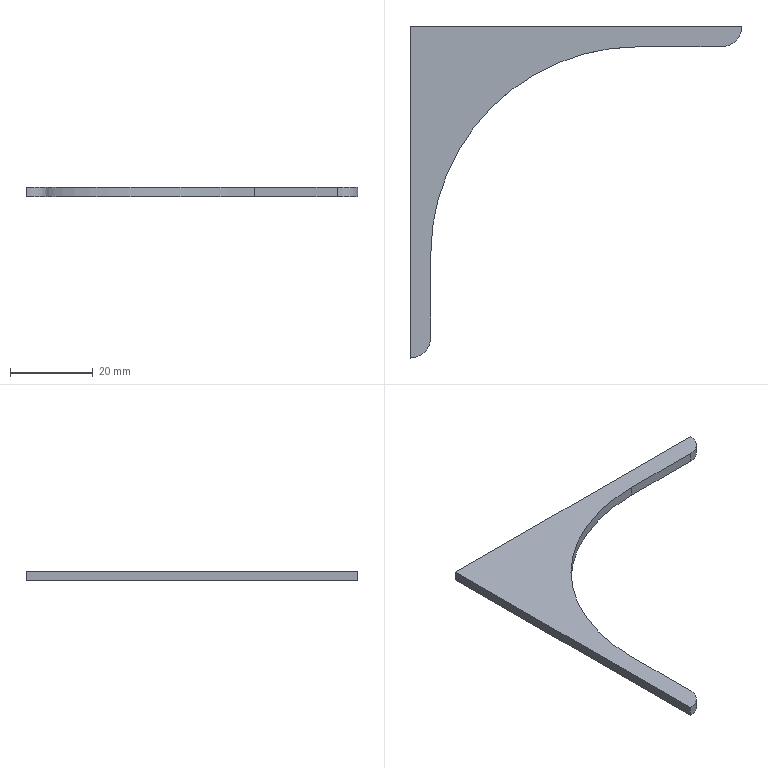Part | SolidWorks | features Fillet 1, FlatPattern 1, SMBaseFlange 1, SheetMetal 1 | 1 solid | 9 faces | box 80 x 80 x 2.3 mm | volume 2992 mm3 | plane 6 | cylinder 3 | commonest cylinder face diameters 10 x2 100 x1
STEP:
#1=CARTESIAN_POINT('',(0.,0.,0.));
#2=VERTEX_POINT('',#1);
#3=CARTESIAN_POINT('',(0.,-80.,0.));
#4=VERTEX_POINT('',#3);
#5=CARTESIAN_POINT('',(0.,0.,0.));
#6=DIRECTION('',(0.,-1.,0.));
#7=VECTOR('',#6,1000.);
#8=LINE('',#5,#7);
#9=EDGE_CURVE('',#2,#4,#8,.T.);
#10=ORIENTED_EDGE('',*,*,#9,.T.);
#11=CARTESIAN_POINT('',(0.,-80.,2.3));
#12=VERTEX_POINT('',#11);
#13=CARTESIAN_POINT('',(0.,-80.,2.3));
#14=DIRECTION('',(0.,0.,-1.));
#15=VECTOR('',#14,1000.);
#16=LINE('',#13,#15);
#17=EDGE_CURVE('',#12,#4,#16,.T.);
#18=ORIENTED_EDGE('',*,*,#17,.F.);
#19=CARTESIAN_POINT('',(0.,0.,2.3));
#20=VERTEX_POINT('',#19);
#21=CARTESIAN_POINT('',(0.,0.,2.3));
#22=DIRECTION('',(0.,-1.,0.));
#23=VECTOR('',#22,1000.);
#24=LINE('',#21,#23);
#25=EDGE_CURVE('',#20,#12,#24,.T.);
#26=ORIENTED_EDGE('',*,*,#25,.F.);
#27=CARTESIAN_POINT('',(0.,0.,2.3));
#28=DIRECTION('',(0.,0.,-1.));
#29=VECTOR('',#28,1000.);
#30=LINE('',#27,#29);
#31=EDGE_CURVE('',#20,#2,#30,.T.);
#32=ORIENTED_EDGE('',*,*,#31,.T.);
#33=EDGE_LOOP('',(#10,#18,#26,#32));
#34=FACE_OUTER_BOUND('',#33,.T.);
#35=CARTESIAN_POINT('',(0.,0.,2.3));
#36=DIRECTION('',(1.,0.,0.));
#37=DIRECTION('',(0.,1.,0.));
#38=AXIS2_PLACEMENT_3D('',#35,#36,#37);
#39=PLANE('',#38);
#40=ADVANCED_FACE('',(#34),#39,.F.);
#41=CARTESIAN_POINT('',(5.,-75.,2.3));
#42=VERTEX_POINT('',#41);
#43=CARTESIAN_POINT('',(5.,-55.,2.3));
#44=VERTEX_POINT('',#43);
#45=CARTESIAN_POINT('',(5.,-80.,2.3));
#46=DIRECTION('',(0.,1.,0.));
#47=VECTOR('',#46,1000.);
#48=LINE('',#45,#47);
#49=EDGE_CURVE('',#42,#44,#48,.T.);
#50=ORIENTED_EDGE('',*,*,#49,.F.);
#51=CARTESIAN_POINT('',(5.,-75.,0.));
#52=VERTEX_POINT('',#51);
#53=CARTESIAN_POINT('',(5.,-75.,2.3));
#54=DIRECTION('',(0.,0.,-1.));
#55=VECTOR('',#54,1000.);
#56=LINE('',#53,#55);
#57=EDGE_CURVE('',#42,#52,#56,.T.);
#58=ORIENTED_EDGE('',*,*,#57,.T.);
#59=CARTESIAN_POINT('',(5.,-55.,0.));
#60=VERTEX_POINT('',#59);
#61=CARTESIAN_POINT('',(5.,-80.,0.));
#62=DIRECTION('',(0.,1.,0.));
#63=VECTOR('',#62,1000.);
#64=LINE('',#61,#63);
#65=EDGE_CURVE('',#52,#60,#64,.T.);
#66=ORIENTED_EDGE('',*,*,#65,.T.);
#67=CARTESIAN_POINT('',(5.,-55.,2.3));
#68=DIRECTION('',(0.,0.,-1.));
#69=VECTOR('',#68,1000.);
#70=LINE('',#67,#69);
#71=EDGE_CURVE('',#44,#60,#70,.T.);
#72=ORIENTED_EDGE('',*,*,#71,.F.);
#73=EDGE_LOOP('',(#50,#58,#66,#72));
#74=FACE_OUTER_BOUND('',#73,.T.);
#75=CARTESIAN_POINT('',(5.,-80.,2.3));
#76=DIRECTION('',(-1.,0.,0.));
#77=DIRECTION('',(0.,-1.,0.));
#78=AXIS2_PLACEMENT_3D('',#75,#76,#77);
#79=PLANE('',#78);
#80=ADVANCED_FACE('',(#74),#79,.F.);
#81=CARTESIAN_POINT('',(55.,-5.,0.));
#82=VERTEX_POINT('',#81);
#83=CARTESIAN_POINT('',(55.,-55.,0.));
#84=DIRECTION('',(0.,0.,-1.));
#85=DIRECTION('',(-1.,0.,0.));
#86=AXIS2_PLACEMENT_3D('',#83,#84,#85);
#87=CIRCLE('',#86,50.);
#88=EDGE_CURVE('',#60,#82,#87,.T.);
#89=ORIENTED_EDGE('',*,*,#88,.T.);
#90=CARTESIAN_POINT('',(55.,-5.,2.3));
#91=VERTEX_POINT('',#90);
#92=CARTESIAN_POINT('',(55.,-5.,2.3));
#93=DIRECTION('',(0.,0.,-1.));
#94=VECTOR('',#93,1000.);
#95=LINE('',#92,#94);
#96=EDGE_CURVE('',#91,#82,#95,.T.);
#97=ORIENTED_EDGE('',*,*,#96,.F.);
#98=CARTESIAN_POINT('',(55.,-55.,2.3));
#99=DIRECTION('',(0.,0.,-1.));
#100=DIRECTION('',(-1.,0.,0.));
#101=AXIS2_PLACEMENT_3D('',#98,#99,#100);
#102=CIRCLE('',#101,50.);
#103=EDGE_CURVE('',#44,#91,#102,.T.);
#104=ORIENTED_EDGE('',*,*,#103,.F.);
#105=ORIENTED_EDGE('',*,*,#71,.T.);
#106=EDGE_LOOP('',(#89,#97,#104,#105));
#107=FACE_OUTER_BOUND('',#106,.T.);
#108=CARTESIAN_POINT('',(55.,-55.,2.3));
#109=DIRECTION('',(0.,0.,-1.));
#110=DIRECTION('',(-1.,0.,0.));
#111=AXIS2_PLACEMENT_3D('',#108,#109,#110);
#112=CYLINDRICAL_SURFACE('',#111,50.);
#113=ADVANCED_FACE('',(#107),#112,.F.);
#114=CARTESIAN_POINT('',(75.,-5.,0.));
#115=VERTEX_POINT('',#114);
#116=CARTESIAN_POINT('',(80.,-5.,0.));
#117=DIRECTION('',(1.,0.,0.));
#118=VECTOR('',#117,1000.);
#119=LINE('',#116,#118);
#120=EDGE_CURVE('',#82,#115,#119,.T.);
#121=ORIENTED_EDGE('',*,*,#120,.T.);
#122=CARTESIAN_POINT('',(75.,-5.,2.3));
#123=VERTEX_POINT('',#122);
#124=CARTESIAN_POINT('',(75.,-5.,2.3));
#125=DIRECTION('',(0.,0.,1.));
#126=VECTOR('',#125,1000.);
#127=LINE('',#124,#126);
#128=EDGE_CURVE('',#115,#123,#127,.T.);
#129=ORIENTED_EDGE('',*,*,#128,.T.);
#130=CARTESIAN_POINT('',(80.,-5.,2.3));
#131=DIRECTION('',(1.,0.,0.));
#132=VECTOR('',#131,1000.);
#133=LINE('',#130,#132);
#134=EDGE_CURVE('',#91,#123,#133,.T.);
#135=ORIENTED_EDGE('',*,*,#134,.F.);
#136=ORIENTED_EDGE('',*,*,#96,.T.);
#137=EDGE_LOOP('',(#121,#129,#135,#136));
#138=FACE_OUTER_BOUND('',#137,.T.);
#139=CARTESIAN_POINT('',(80.,-5.,2.3));
#140=DIRECTION('',(0.,1.,0.));
#141=DIRECTION('',(-1.,0.,0.));
#142=AXIS2_PLACEMENT_3D('',#139,#140,#141);
#143=PLANE('',#142);
#144=ADVANCED_FACE('',(#138),#143,.F.);
#145=CARTESIAN_POINT('',(80.,0.,0.));
#146=VERTEX_POINT('',#145);
#147=CARTESIAN_POINT('',(0.,0.,0.));
#148=DIRECTION('',(-1.,0.,0.));
#149=VECTOR('',#148,1000.);
#150=LINE('',#147,#149);
#151=EDGE_CURVE('',#146,#2,#150,.T.);
#152=ORIENTED_EDGE('',*,*,#151,.T.);
#153=ORIENTED_EDGE('',*,*,#31,.F.);
#154=CARTESIAN_POINT('',(80.,0.,2.3));
#155=VERTEX_POINT('',#154);
#156=CARTESIAN_POINT('',(0.,0.,2.3));
#157=DIRECTION('',(-1.,0.,0.));
#158=VECTOR('',#157,1000.);
#159=LINE('',#156,#158);
#160=EDGE_CURVE('',#155,#20,#159,.T.);
#161=ORIENTED_EDGE('',*,*,#160,.F.);
#162=CARTESIAN_POINT('',(80.,0.,2.3));
#163=DIRECTION('',(0.,0.,-1.));
#164=VECTOR('',#163,1000.);
#165=LINE('',#162,#164);
#166=EDGE_CURVE('',#155,#146,#165,.T.);
#167=ORIENTED_EDGE('',*,*,#166,.T.);
#168=EDGE_LOOP('',(#152,#153,#161,#167));
#169=FACE_OUTER_BOUND('',#168,.T.);
#170=CARTESIAN_POINT('',(0.,0.,2.3));
#171=DIRECTION('',(0.,-1.,0.));
#172=DIRECTION('',(0.,0.,-1.));
#173=AXIS2_PLACEMENT_3D('',#170,#171,#172);
#174=PLANE('',#173);
#175=ADVANCED_FACE('',(#169),#174,.F.);
#176=ORIENTED_EDGE('',*,*,#134,.T.);
#177=CARTESIAN_POINT('',(75.,0.,2.3));
#178=DIRECTION('',(0.,0.,1.));
#179=DIRECTION('',(-1.,0.,0.));
#180=AXIS2_PLACEMENT_3D('',#177,#178,#179);
#181=CIRCLE('',#180,5.);
#182=EDGE_CURVE('',#123,#155,#181,.T.);
#183=ORIENTED_EDGE('',*,*,#182,.T.);
#184=ORIENTED_EDGE('',*,*,#160,.T.);
#185=ORIENTED_EDGE('',*,*,#25,.T.);
#186=CARTESIAN_POINT('',(0.,-75.,2.3));
#187=DIRECTION('',(0.,0.,1.));
#188=DIRECTION('',(-1.,0.,0.));
#189=AXIS2_PLACEMENT_3D('',#186,#187,#188);
#190=CIRCLE('',#189,5.);
#191=EDGE_CURVE('',#12,#42,#190,.T.);
#192=ORIENTED_EDGE('',*,*,#191,.T.);
#193=ORIENTED_EDGE('',*,*,#49,.T.);
#194=ORIENTED_EDGE('',*,*,#103,.T.);
#195=EDGE_LOOP('',(#176,#183,#184,#185,#192,#193,#194));
#196=FACE_OUTER_BOUND('',#195,.T.);
#197=CARTESIAN_POINT('',(55.,-55.,2.3));
#198=DIRECTION('',(0.,0.,-1.));
#199=DIRECTION('',(-1.,0.,0.));
#200=AXIS2_PLACEMENT_3D('',#197,#198,#199);
#201=PLANE('',#200);
#202=ADVANCED_FACE('',(#196),#201,.F.);
#203=ORIENTED_EDGE('',*,*,#151,.F.);
#204=CARTESIAN_POINT('',(75.,0.,0.));
#205=DIRECTION('',(0.,0.,-1.));
#206=DIRECTION('',(-1.,0.,0.));
#207=AXIS2_PLACEMENT_3D('',#204,#205,#206);
#208=CIRCLE('',#207,5.);
#209=EDGE_CURVE('',#146,#115,#208,.T.);
#210=ORIENTED_EDGE('',*,*,#209,.T.);
#211=ORIENTED_EDGE('',*,*,#120,.F.);
#212=ORIENTED_EDGE('',*,*,#88,.F.);
#213=ORIENTED_EDGE('',*,*,#65,.F.);
#214=CARTESIAN_POINT('',(0.,-75.,0.));
#215=DIRECTION('',(0.,0.,-1.));
#216=DIRECTION('',(-1.,0.,0.));
#217=AXIS2_PLACEMENT_3D('',#214,#215,#216);
#218=CIRCLE('',#217,5.);
#219=EDGE_CURVE('',#52,#4,#218,.T.);
#220=ORIENTED_EDGE('',*,*,#219,.T.);
#221=ORIENTED_EDGE('',*,*,#9,.F.);
#222=EDGE_LOOP('',(#203,#210,#211,#212,#213,#220,#221));
#223=FACE_OUTER_BOUND('',#222,.T.);
#224=CARTESIAN_POINT('',(55.,-55.,0.));
#225=DIRECTION('',(0.,0.,-1.));
#226=DIRECTION('',(-1.,0.,0.));
#227=AXIS2_PLACEMENT_3D('',#224,#225,#226);
#228=PLANE('',#227);
#229=ADVANCED_FACE('',(#223),#228,.T.);
#230=ORIENTED_EDGE('',*,*,#182,.F.);
#231=ORIENTED_EDGE('',*,*,#128,.F.);
#232=ORIENTED_EDGE('',*,*,#209,.F.);
#233=ORIENTED_EDGE('',*,*,#166,.F.);
#234=EDGE_LOOP('',(#230,#231,#232,#233));
#235=FACE_OUTER_BOUND('',#234,.T.);
#236=CARTESIAN_POINT('',(75.,0.,2.3));
#237=DIRECTION('',(0.,0.,-1.));
#238=DIRECTION('',(-1.,0.,0.));
#239=AXIS2_PLACEMENT_3D('',#236,#237,#238);
#240=CYLINDRICAL_SURFACE('',#239,5.);
#241=ADVANCED_FACE('',(#235),#240,.T.);
#242=ORIENTED_EDGE('',*,*,#191,.F.);
#243=ORIENTED_EDGE('',*,*,#17,.T.);
#244=ORIENTED_EDGE('',*,*,#219,.F.);
#245=ORIENTED_EDGE('',*,*,#57,.F.);
#246=EDGE_LOOP('',(#242,#243,#244,#245));
#247=FACE_OUTER_BOUND('',#246,.T.);
#248=CARTESIAN_POINT('',(0.,-75.,2.3));
#249=DIRECTION('',(0.,0.,-1.));
#250=DIRECTION('',(-1.,0.,0.));
#251=AXIS2_PLACEMENT_3D('',#248,#249,#250);
#252=CYLINDRICAL_SURFACE('',#251,5.);
#253=ADVANCED_FACE('',(#247),#252,.T.);
#254=CLOSED_SHELL('',(#40,#80,#113,#144,#175,#202,#229,#241,#253));
#255=MANIFOLD_SOLID_BREP('',#254);
#256=CARTESIAN_POINT('',(0.,0.,0.));
#257=DIRECTION('',(0.,0.,1.));
#258=DIRECTION('',(1.,0.,0.));
#259=AXIS2_PLACEMENT_3D('',#256,#257,#258);
#260=(LENGTH_UNIT()NAMED_UNIT(*)SI_UNIT(.MILLI.,.METRE.));
#261=UNCERTAINTY_MEASURE_WITH_UNIT(LENGTH_MEASURE(0.00001),#260,'','');
#262=(NAMED_UNIT(*)PLANE_ANGLE_UNIT()SI_UNIT($,.RADIAN.));
#263=(NAMED_UNIT(*)SI_UNIT($,.STERADIAN.)SOLID_ANGLE_UNIT());
#264=(GEOMETRIC_REPRESENTATION_CONTEXT(3)GLOBAL_UNCERTAINTY_ASSIGNED_CONTEXT((#261))GLOBAL_UNIT_ASSIGNED_CONTEXT((#260,#262,#263))REPRESENTATION_CONTEXT('',''));
#265=ADVANCED_BREP_SHAPE_REPRESENTATION('',(#255,#259),#264);